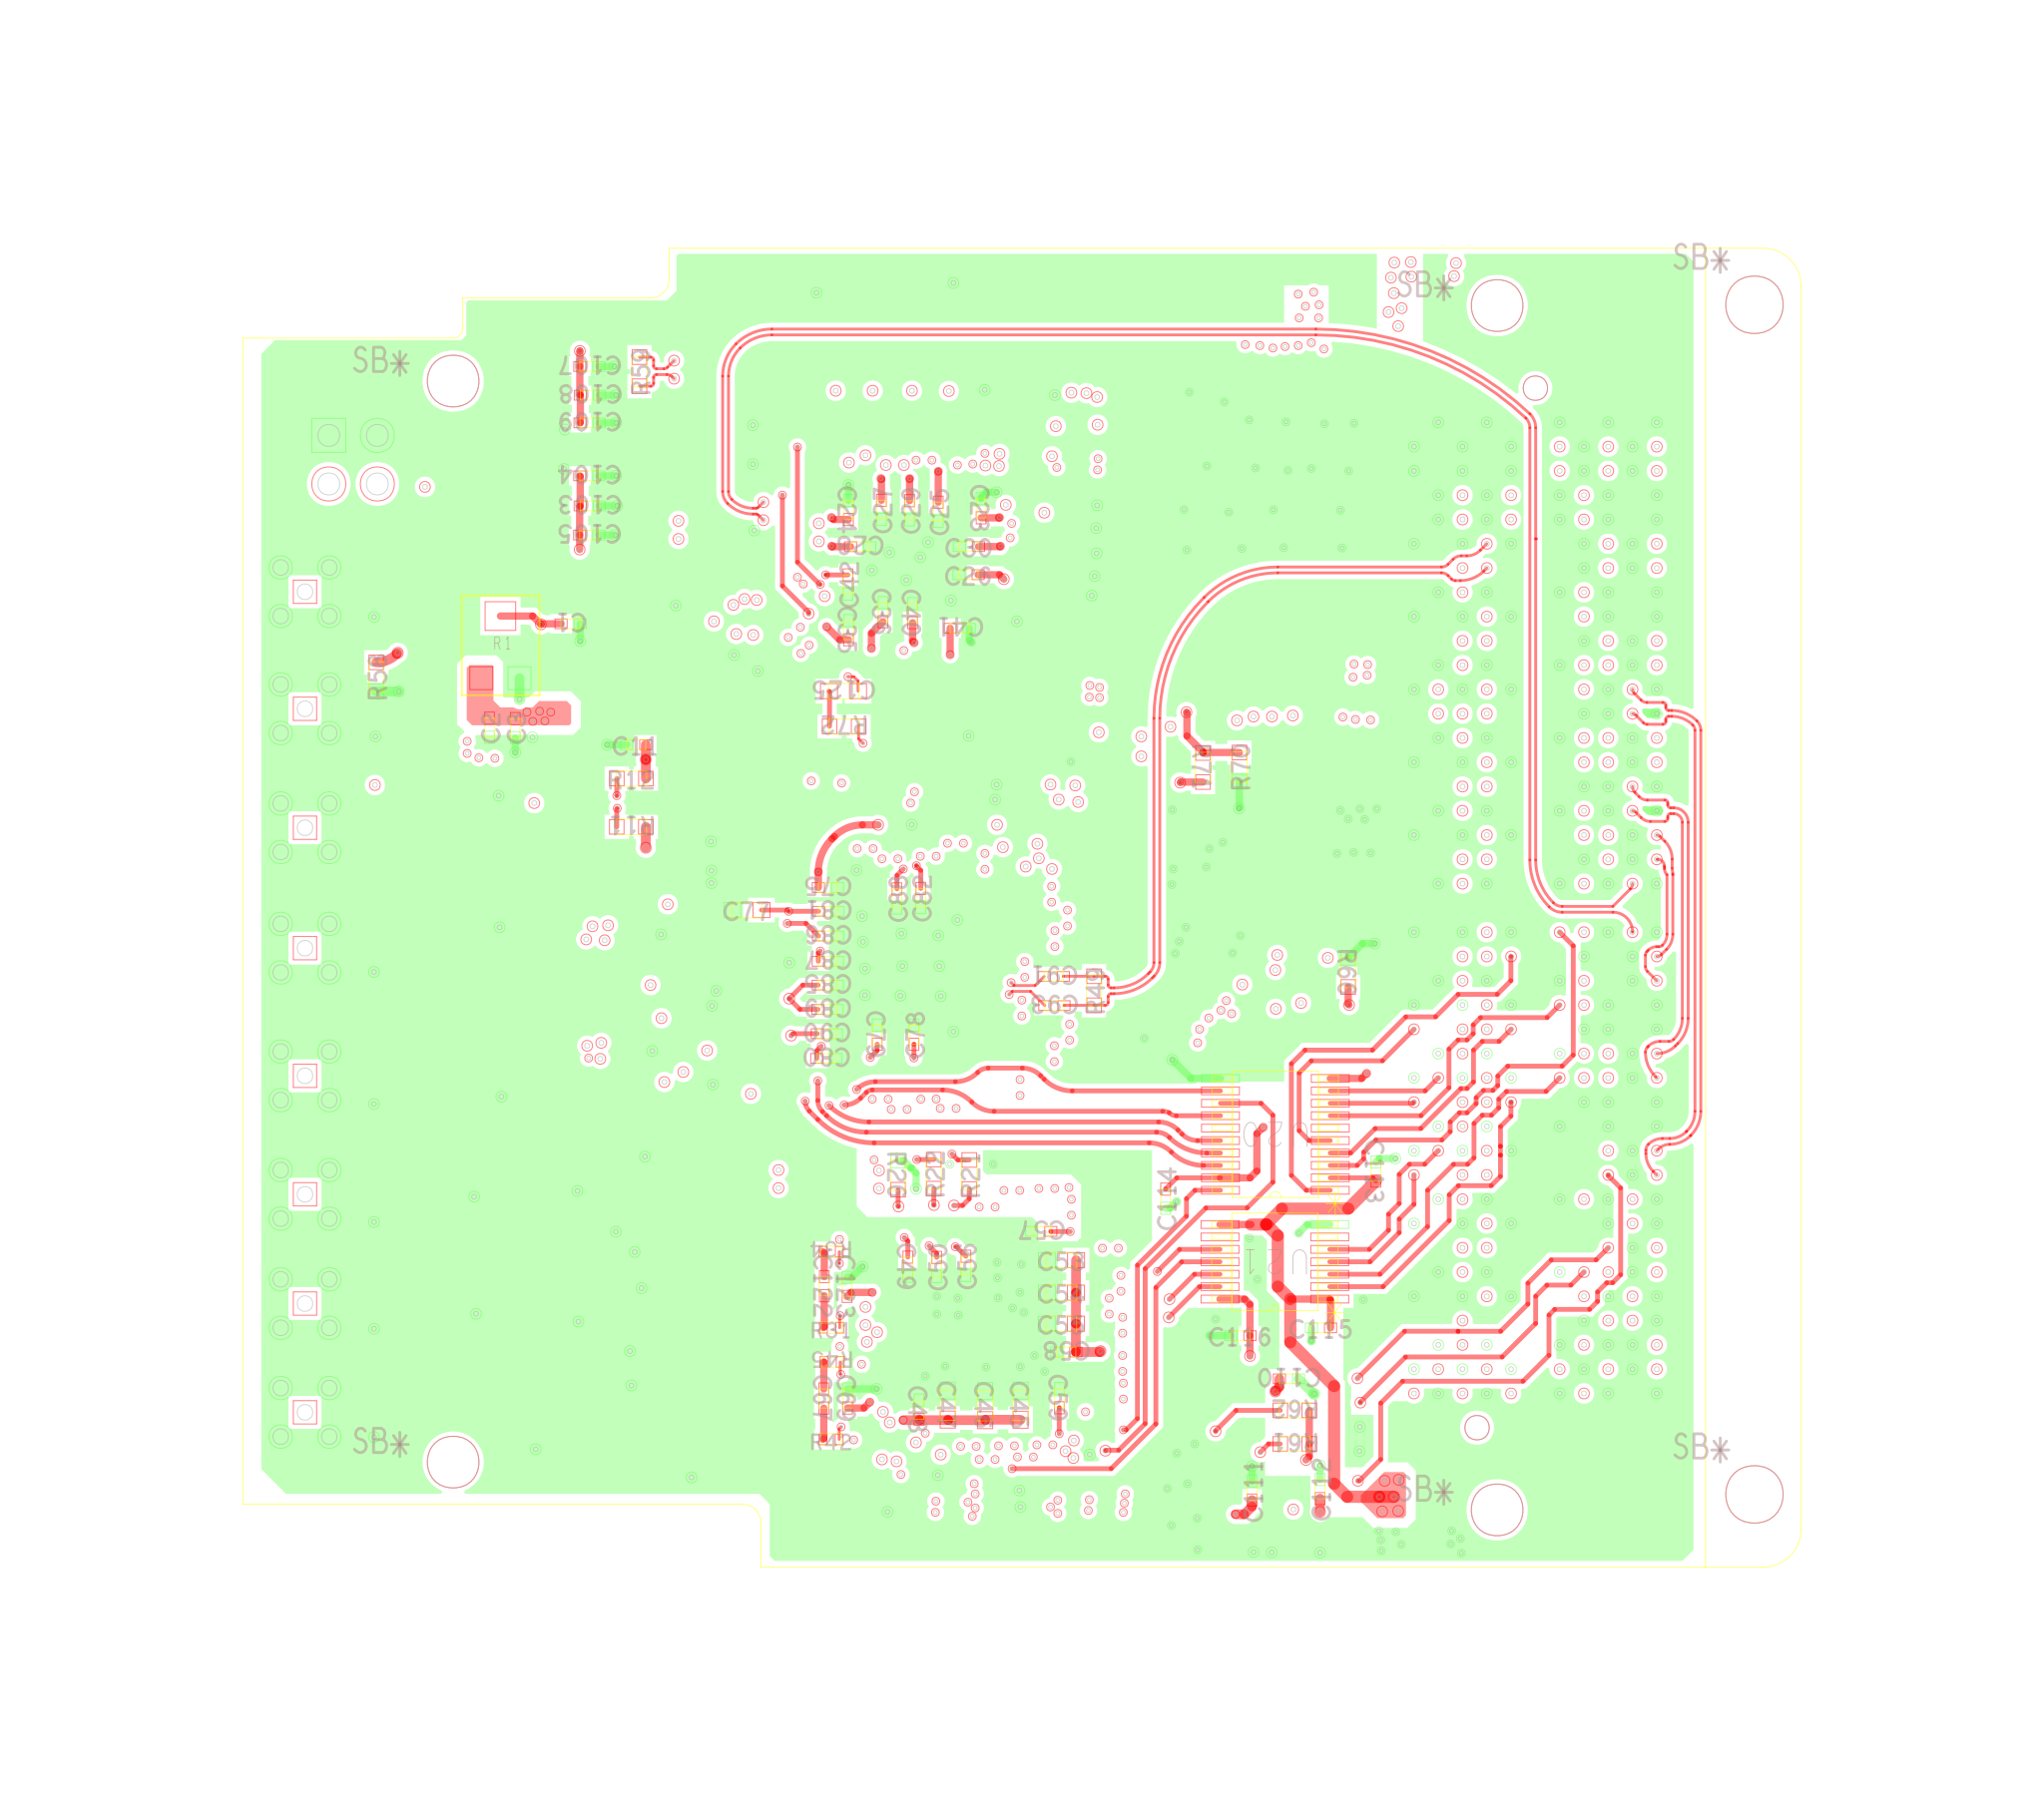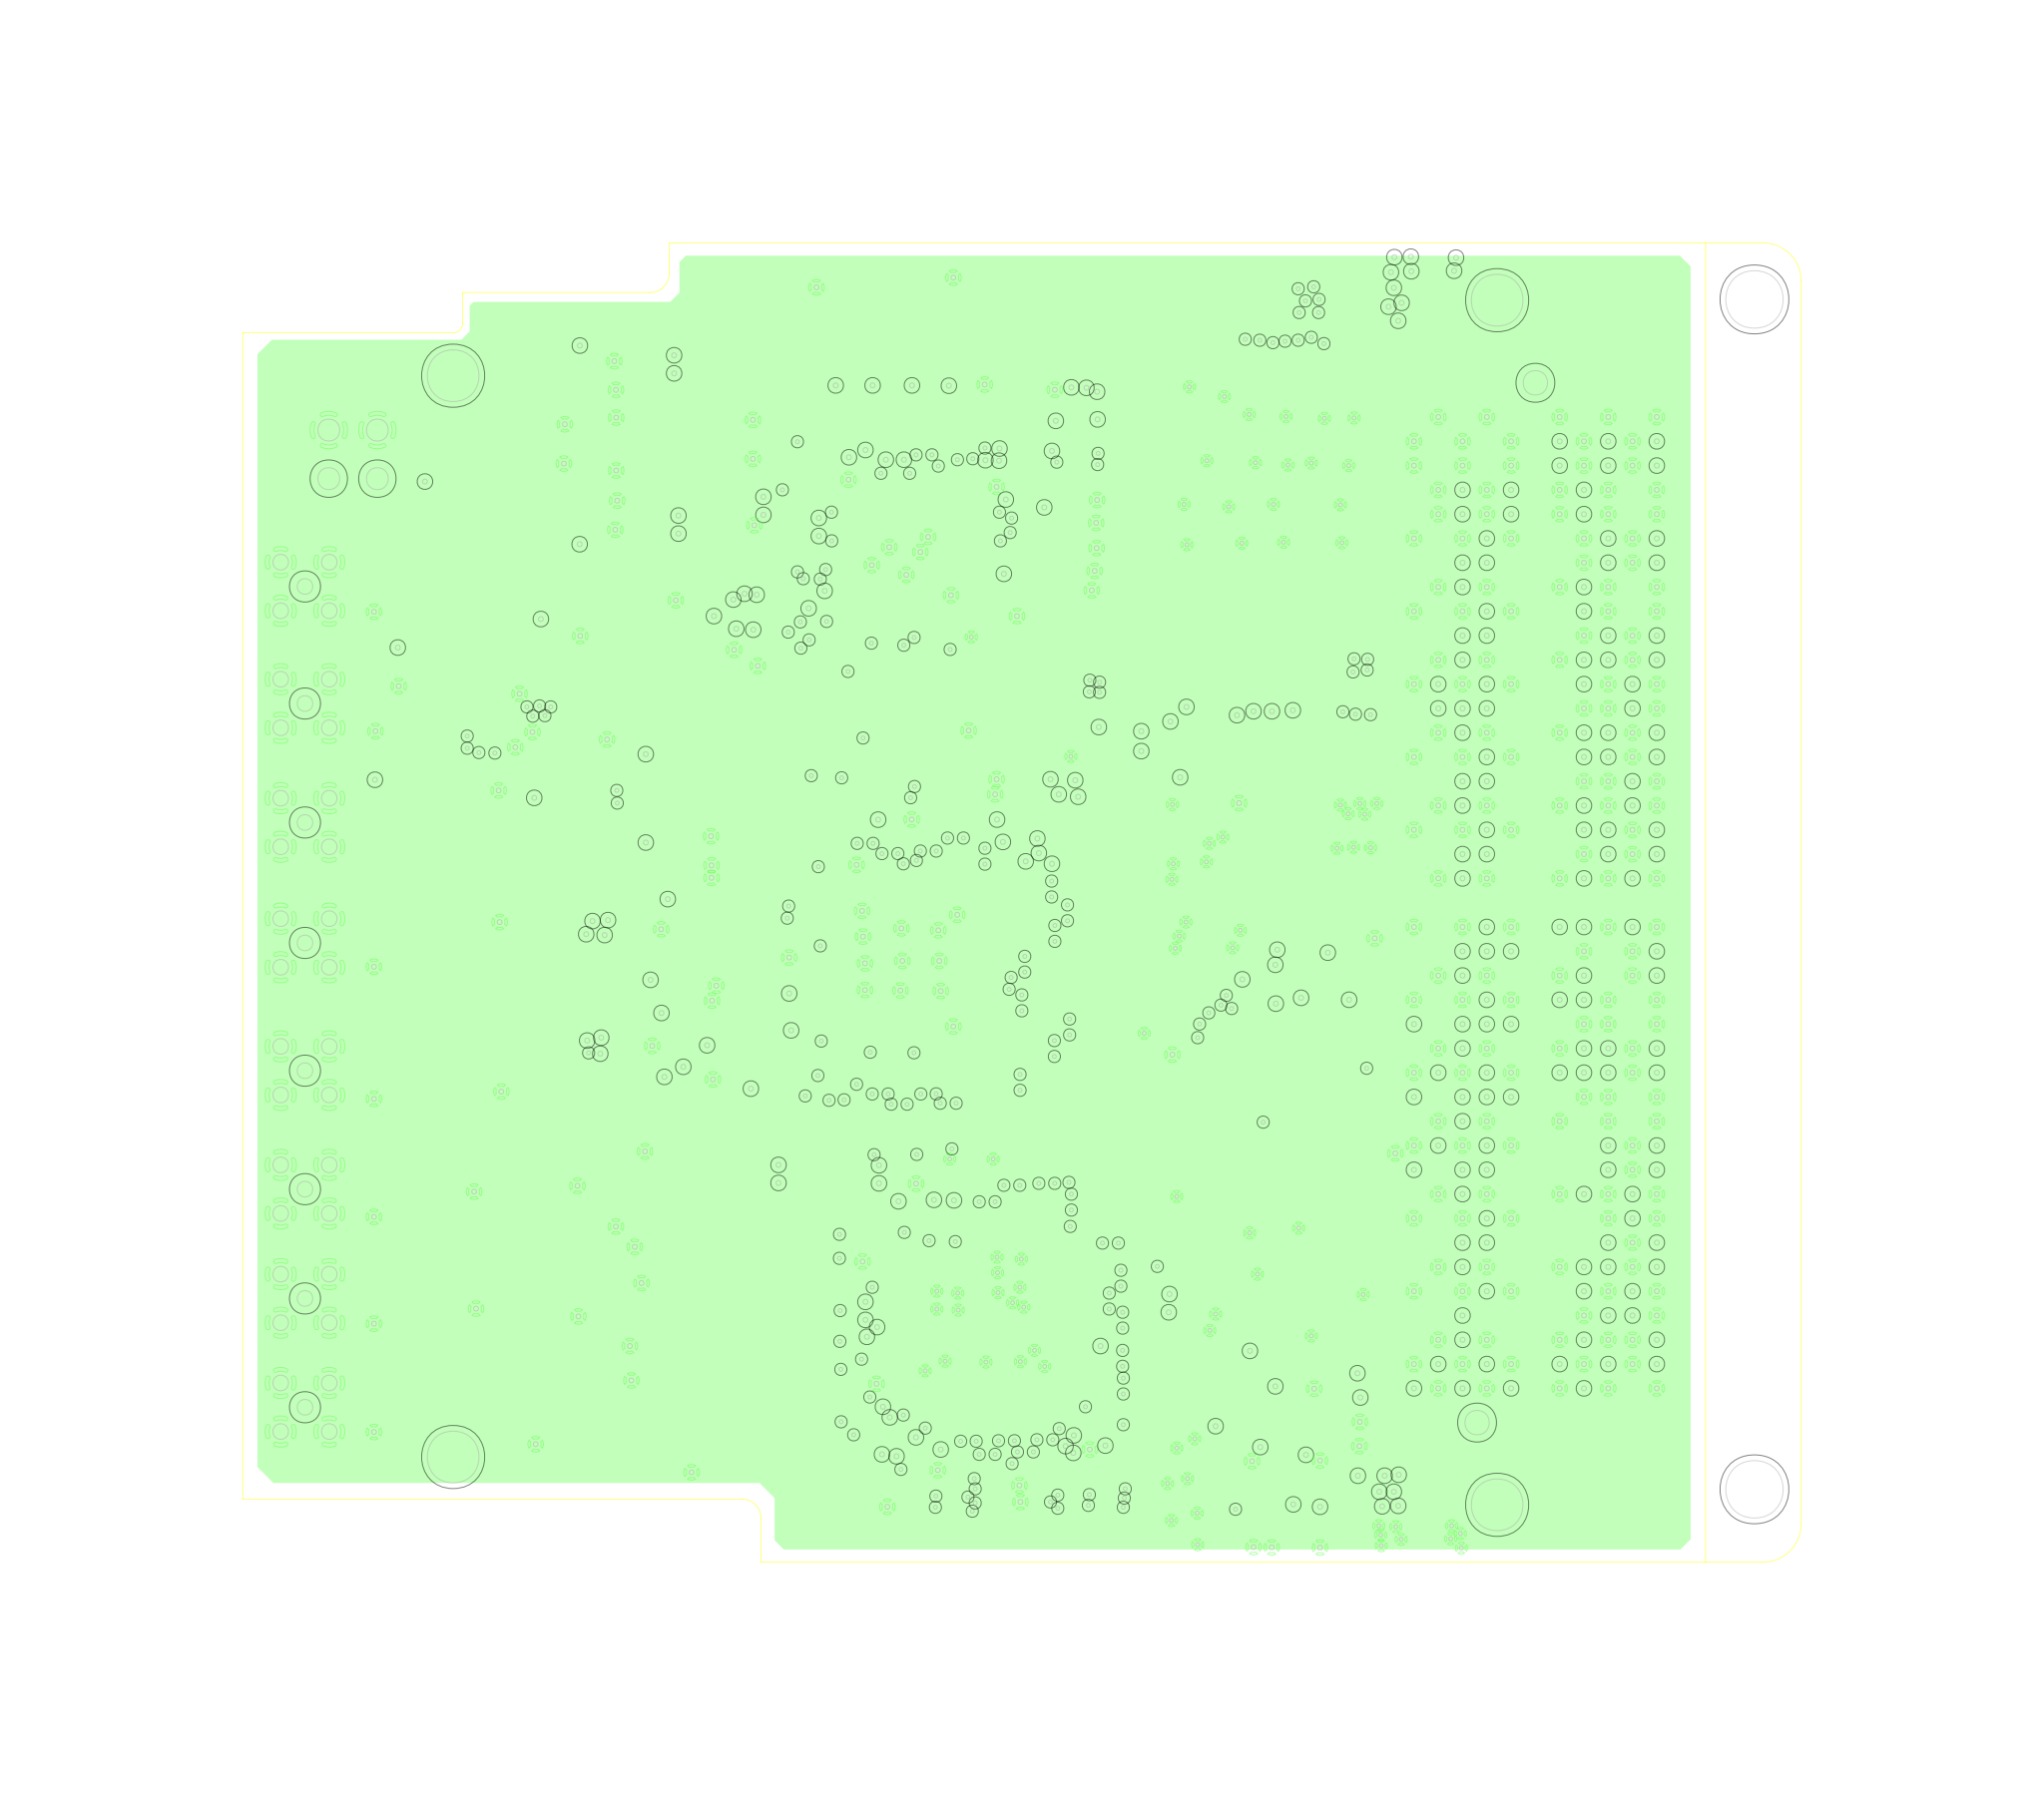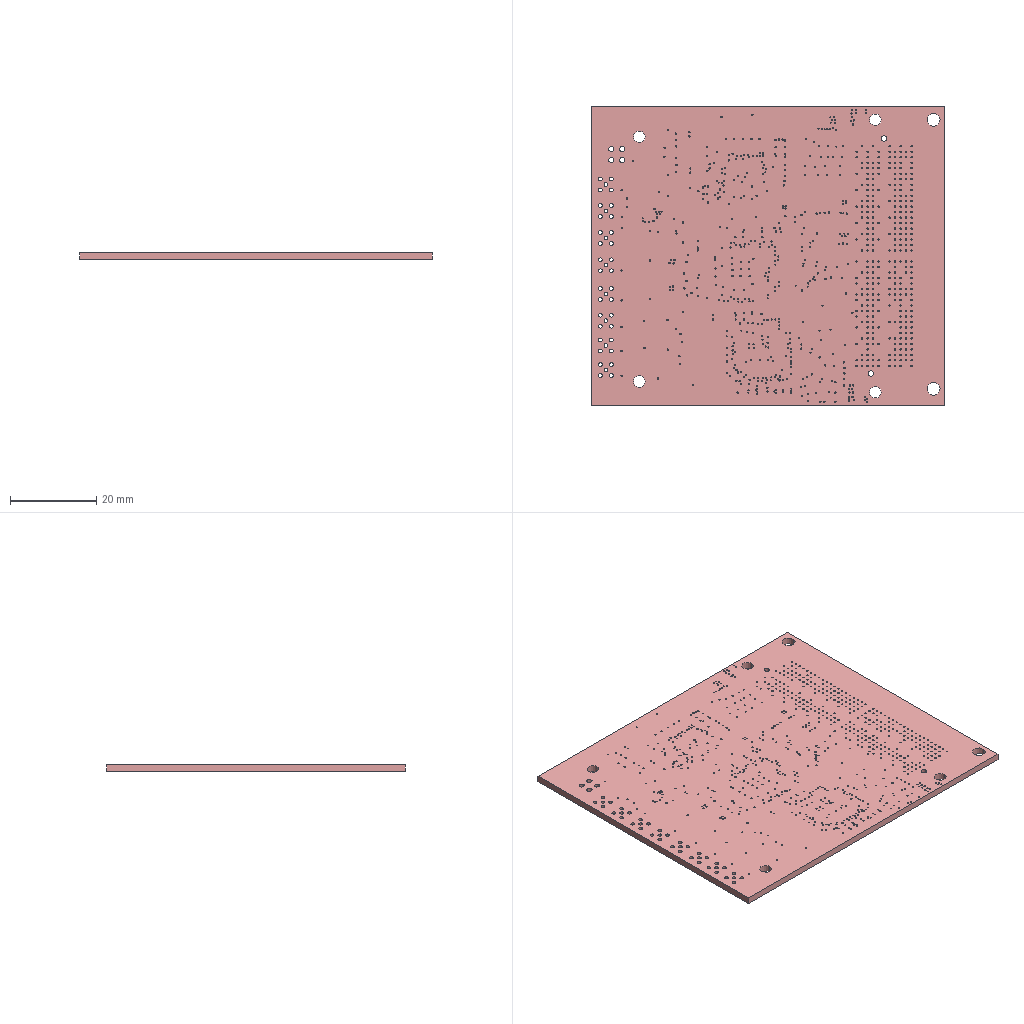Circuit board layout | Cadence Allegro | box 81.5 x 69 x 1.6 mm
Layer stack:
# Cadence Allegro layer stack of  (unit mm; from the constraint file cross-section; dielectric type: 0 not recorded (Allegro does not mark core vs prepreg), 3 surface material)
index,name,kind,layer,copper_thickness_mm,dielectric_type,dielectric_thickness_mm,dielectric_material,dielectric_constant
0,Top Surface,other,,,,,,
1,TOP,copper,TOP,0.0305,,,,
2,Dielectric1,dielectric,,,0,0.2032,FR-4,4.5
3,GND02,copper,GND02,0.0305,,,,
4,Dielectric2,dielectric,,,0,0.2032,FR-4,4.5
5,ART03,copper,ART03,0.0305,,,,
6,Dielectric3,dielectric,,,0,0.2032,FR-4,4.5
7,GND04,copper,GND04,0.0305,,,,
8,Dielectric4,dielectric,,,0,0.2032,FR-4,4.5
9,PWR05,copper,PWR05,0.0305,,,,
10,Dielectric5,dielectric,,,0,0.2032,FR-4,4.5
11,ART06,copper,ART06,0.0305,,,,
12,Dielectric6,dielectric,,,0,0.2032,FR-4,4.5
13,GND07,copper,GND07,0.0305,,,,
14,Dielectric7,dielectric,,,0,0.2032,FR-4,4.5
15,BOTTOM,copper,BOTTOM,0.0305,,,,
16,Bottom Surface,other,,,,,,
# drill layer pairs: low layer,high layer
drill_pair,TOP,BOTTOM
Part placement:
REFDES,COMP_VALUE,SYM_NAME,SYM_X,SYM_Y,SYM_ROTATE,SYM_MIRROR
C1,100nF,FPC-0402C,2831.000,3523.000,180.000,NO
C2,1uF,FPC-0402C,2664.000,3309.000,90.000,NO
C3,100nF,FPC-0402C,2717.000,3308.000,90.000,NO
C4,10nF,FPC-0402C,2716.000,3309.000,270.000,YES
C10,100nF,FPC-0402C,2426.240,2935.189,270.000,YES
C11,100nF,FPC-0402C,2966.000,3274.000,0.000,NO
C12,10uF,FPC-0603C,3650.559,3358.776,90.000,YES
C13,10uF,FPC-0603C,3236.177,3890.441,0.000,YES
C14,1uF,FPC-0402C,3236.177,3388.083,0.000,YES
C15,100nF,FPC-0402C,2954.913,3104.917,180.000,YES
C18,100nF,FPC-0402C,2957.181,3200.917,180.000,YES
C19,100nF,FPC-0402C,2426.240,3122.441,90.000,YES
C20,10uF,FPC-0603C,3836.142,3784.441,0.000,YES
C21,47uF,FPC-1206C,3766.240,3920.307,270.000,YES
C22,10uF,FPC-0603C,3683.559,3941.394,90.000,YES
C23,100nF,FPC-0402C,3676.083,3760.953,270.000,NO
C24,100nF,FPC-0402C,3403.083,3757.575,270.000,NO
C25,100nF,FPC-0402C,3587.917,3753.803,90.000,NO
C26,100nF,FPC-0402C,3650.315,3624.083,0.000,NO
C27,100nF,FPC-0402C,3470.917,3757.717,90.000,NO
C28,100nF,FPC-0402C,3427.063,3681.917,180.000,NO
C29,100nF,FPC-0402C,3528.917,3756.850,90.000,NO
C30,100nF,FPC-0402C,3651.071,3682.083,0.000,NO
C31,10uF,FPC-0603C,3836.142,3447.441,0.000,YES
C32,100nF,FPC-0402C,3834.142,3560.083,0.000,YES
C33,100nF,FPC-0402C,3834.142,3508.083,0.000,YES
C34,10uF,FPC-0603C,3239.177,3458.559,180.000,YES
C35,100nF,FPC-0402C,3403.083,3509.823,270.000,NO
C36,100nF,FPC-0402C,3474.000,3547.000,270.000,NO
C37,1uF,FPC-0603C,3393.980,3384.740,0.000,YES
C38,10nF,FPC-0603C,3535.823,3420.260,180.000,YES
C39,10uF,FPC-0603C,3239.177,3683.559,180.000,YES
C40,100nF,FPC-0402C,3535.083,3545.039,270.000,NO
C41,100nF,FPC-0402C,3632.055,3513.917,180.000,NO
C42,100nF,FPC-0402C,3401.917,3603.992,90.000,NO
C43,10uF,FPC-0603C,3618.559,1739.516,90.000,YES
C44,100nF,FPC-0402C,3483.083,1749.094,270.000,YES
C45,10uF,FPC-0603C,3757.441,1913.673,270.000,NO
C46,10uF,FPC-0603C,3684.441,1912.831,270.000,NO
C47,10uF,FPC-0603C,3607.441,1913.988,270.000,NO
C48,10nF,FPC-0402C,3548.240,1904.433,270.000,NO
C49,10nF,FPC-0402C,3525.240,2199.008,270.000,NO
C50,10nF,FPC-0402C,3584.760,2198.370,90.000,NO
C51,10uF,FPC-0603C,3934.559,1738.146,90.000,YES
C52,100nF,FPC-0402C,3788.083,1748.472,270.000,YES
C53,10uF,FPC-0603C,3841.697,2212.441,0.000,NO
C54,10uF,FPC-0603C,3841.539,2145.441,0.000,NO
C55,10uF,FPC-0603C,3841.382,2081.441,0.000,NO
C56,10nF,FPC-0402C,3644.760,2200.748,90.000,NO
C57,10nF,FPC-0402C,3799.874,2271.760,180.000,NO
C58,10nF,FPC-0402C,3851.496,2023.260,180.000,NO
C59,10nF,FPC-0402C,3837.240,1928.118,270.000,NO
C60,100nF,FPC-0402C,2426.240,2198.748,270.000,YES
C61,100nF,FPC-0402C,3292.083,2105.228,270.000,YES
C62,100nF,FPC-0402C,3291.917,2200.811,90.000,YES
C63,100nF,FPC-0402C,2904.433,2300.083,0.000,YES
C64,100nF,FPC-0402C,2904.016,2354.917,180.000,YES
C65,100nF,FPC-0402C,2426.240,1976.323,270.000,YES
C66,100nF,FPC-0402C,3293.083,1876.701,270.000,YES
C67,3.3pF,FPC-0402C,3352.240,1927.433,270.000,NO
C68,100nF,FPC-0402C,3292.917,1971.921,90.000,YES
C69,100nF,FPC-0402C,3401.083,1927.543,270.000,NO
C70,100nF,FPC-0402C,2896.165,2025.083,0.000,YES
C71,100nF,FPC-0402C,2896.213,2085.917,180.000,YES
C72,100nF,FPC-0402C,3406.409,2349.083,0.000,YES
C73,100nF,FPC-0402C,3407.031,2408.083,0.000,YES
C74,10uF,FPC-0603C,3569.441,3139.122,270.000,YES
C75,100nF,FPC-0402C,3360.654,2979.917,180.000,NO
C76,47uF,FPC-1206C,3172.504,2933.240,0.000,YES
C77,10uF,FPC-0603C,3193.965,2933.441,0.000,NO
C78,100nF,FPC-0402C,3537.917,2676.724,90.000,NO
C79,100nF,FPC-0402C,3462.083,2676.898,270.000,NO
C80,100nF,FPC-0402C,3357.520,2627.917,180.000,NO
C81,100nF,FPC-0402C,3361.142,2930.917,180.000,NO
C82,100nF,FPC-0402C,3551.917,2958.236,90.000,NO
C83,10uF,FPC-0603C,3744.559,3139.193,90.000,YES
C84,10uF,FPC-0603C,3671.559,3139.350,90.000,YES
C85,100nF,FPC-0402C,3360.386,2778.917,180.000,NO
C86,100nF,FPC-0402C,3361.126,2880.059,180.000,NO
C87,100nF,FPC-0402C,3360.630,2827.917,180.000,NO
C88,100nF,FPC-0402C,3502.760,2957.378,90.000,NO
C89,100nF,FPC-0402C,3359.874,2728.917,180.000,NO
C90,100nF,FPC-0402C,3358.496,2678.917,180.000,NO
C91,10nF,FPC-0402C,3825.740,2796.760,180.000,NO
C92,10nF,FPC-0402C,3327.240,3150.638,270.000,YES
C93,10nF,FPC-0402C,3826.984,2736.760,180.000,NO
C94,10nF,FPC-0402C,3387.240,3147.394,270.000,YES
C95,100nF,FPC-0402C,3180.118,2736.083,0.000,YES
C96,100nF,FPC-0402C,2426.240,2424.260,270.000,YES
C97,1nF,FPC-0402C,3171.008,3014.760,180.000,YES
C98,150nF,FPC-0402C,3170.772,3074.760,180.000,YES
C99,100nF,FPC-0402C,2941.362,2643.083,0.000,YES
C100,100nF,FPC-0402C,2426.240,2672.591,270.000,YES
C101,100nF,FPC-0402C,2957.787,2883.240,0.000,YES
C102,100nF,FPC-0402C,2429.760,3426.165,90.000,YES
C103,1uF,FPC-0402C,2870.386,3765.760,180.000,NO
C104,100nF,FPC-0402C,2869.543,3827.760,180.000,NO
C105,100nF,FPC-0402C,2869.244,3705.760,180.000,NO
C106,100nF,FPC-0402C,2426.240,3664.701,270.000,YES
C107,1uF,FPC-0402C,2869.606,4052.917,180.000,NO
C108,100nF,FPC-0402C,2870.677,3993.760,180.000,NO
C109,100nF,FPC-0402C,2870.055,3936.760,180.000,NO
C110,100nF,FPC-0402C,4310.000,1968.000,180.000,NO
C111,100nF,FPC-0402C,4234.000,1738.000,90.000,NO
C112,100nF,FPC-0402C,4374.000,1741.000,90.000,NO
C113,100nF,FPC-0402C,4489.000,2395.000,270.000,NO
C114,100nF,FPC-0402C,4056.000,2339.000,90.000,NO
C115,100nF,FPC-0402C,4376.000,2073.000,0.000,NO
C116,100nF,FPC-0402C,4210.000,2057.000,0.000,NO
C117,100uF,FPC-3528T,4184.000,4187.000,0.000,YES
C118,330uF,FPC-7343T,4303.000,3100.000,90.000,YES
C119,10uF,FPC-0603C,4150.000,2799.000,90.000,YES
C120,33pF,FPC-0402C,4336.000,2811.000,270.000,YES
C121,10uF,FPC-0603C,4246.000,2801.000,90.000,YES
C122,3.3pF,FPC-0402C,3353.240,2158.811,270.000,NO
C123,100nF,FPC-0402C,3400.083,2157.465,270.000,NO
C124,10uF,FPC-0603C,4459.000,3219.000,270.000,YES
C125,1uF,FPC-0603C,3392.823,3384.260,180.000,NO
C126,1nF,FPC-0402C,3182.370,2581.240,0.000,YES
C127,47uF,FPC-1206C,4144.000,3191.000,90.000,YES
C128,47uF,FPC-1206C,4594.000,1696.000,90.000,YES
C129,10nF,FPC-0603C,3535.823,3354.260,180.000,YES
C130,1nF,FPC-1206C,3559.000,4162.000,0.000,YES
C134,1nF,FPC-1206C,3020.000,1823.000,0.000,YES
D2,533-0121F,FPC-LED4-4R3X8R1-1R1-1,2383.000,3861.000,90.000,YES
D3,PESD3V3X1BL,SOD882,2426.043,2828.339,270.000,YES
D4,PESD3V3X1BL,SOD882,2426.043,2096.535,270.000,YES
D5,PESD3V3X1BL,SOD882,2426.043,1872.559,270.000,YES
D6,PESD3V3X1BL,SOD882,2426.043,2320.583,270.000,YES
D7,PESD3V3X1BL,SOD882,2426.043,2566.606,270.000,YES
D8,PESD3V3X1BL,SOD882,2429.000,3321.000,270.000,YES
D9,PESD3V3X1BL,SOD882,2426.043,3561.654,270.000,YES
J1,CON-MMCX-Angle,SMA,2284.000,2855.000,0.000,YES
J2,CON-MMCX,SMA,2284.000,3103.000,0.000,YES
J3,CON-MMCX-Angle,SMA,2284.000,2123.000,0.000,YES
J4,CON-MMCX-Angle,SMA,2284.000,1899.000,0.000,YES
J5,CON-MMCX-Angle,SMA,2284.000,2348.000,0.000,YES
J6,CON-MMCX-Angle,SMA,2284.000,2592.000,0.000,YES
J7,CON-MMCX-Angle,SMA,2284.000,3348.000,0.000,YES
J8,CON-MMCX-Angle,SMA,2284.000,3589.000,0.000,YES
J9,ASP-134485-01,FPC-CON90VP1R27-10X40SM,4817.421,2937.870,270.000,YES
L1,BLM18HE152SN1,FPC-0603L,2647.000,3309.000,270.000,YES
L2,BLM18HE152SN1,FPC-0603L,3836.142,3377.240,0.000,YES
L3,BLM18HE152SN1,FPC-0603L,3239.177,3530.760,180.000,YES
L4,BLM18HE152SN1,FPC-0603L,3239.177,3609.760,180.000,YES
L6,BLM18HE152SN1,FPC-0603L,3494.760,3138.858,90.000,YES
L12,BLM18EG221SN1,FPC-0603L,3843.858,3109.240,0.000,YES
L13,BLM18EG221SN1,FPC-0603L,3548.240,1739.142,270.000,YES
L14,BLM18HE152SN1,FPC-0603L,3862.240,1738.142,270.000,YES
L15,BLM18EG221SN1,FPC-0603L,3871.760,3889.858,90.000,YES
R1,10K,VR5,2647.000,3411.000,0.000,NO
R2,33R,FPC-0603R,3126.000,3451.000,270.000,YES
R3,4.7K,FPC-0603R,2850.000,3313.000,180.000,YES
R11,121R,FPC-0603R,2955.835,3104.760,180.000,NO
R12,121R,FPC-0603R,2956.008,3204.240,0.000,NO
R13,NC_10K,FPC-0603R,3836.142,3627.240,0.000,YES
R14,4.7K,FPC-0603R,3452.760,3941.394,90.000,YES
R15,1K,FPC-0603R,3376.760,3941.394,90.000,YES
R16,1K,FPC-0603R,3836.142,3704.240,0.000,YES
R17,33R,FPC-0603R,3609.760,3941.394,90.000,YES
R18,200R,FPC-0603R,3835.291,3310.760,180.000,YES
R19,4.7K,FPC-0603R,3533.760,3941.394,90.000,YES
R20,10K,FPC-0603R,3393.866,3311.240,0.000,YES
R21,NC_0R,FPC-0603R,3651.760,2388.819,90.000,NO
R22,NC_0R,FPC-0603R,3578.760,2389.661,90.000,NO
R23,NC_0R,FPC-0603R,3505.240,2388.504,270.000,YES
R24,0R,FPC-0603R,3650.760,2389.126,90.000,YES
R25,0R,FPC-0603R,3577.760,2390.283,90.000,YES
R26,0R,FPC-0603R,3505.240,2387.441,270.000,NO
R28,5R,FPC-0402R,3369.209,2124.760,180.000,YES
R29,NC_49.9R,FPC-0603R,2897.772,2229.240,0.000,YES
R30,24.9R,FPC-0402R,3368.594,2072.240,0.000,YES
R31,49.9R,FPC-0402R,3368.232,2073.240,0.000,NO
R32,NC_49.9R,FPC-0603R,2903.071,2425.760,180.000,YES
R33,24.9R,FPC-0402R,3367.862,2229.760,180.000,YES
R34,49.9R,FPC-0402R,3367.311,2229.760,180.000,NO
R36,5R,FPC-0402R,3367.665,2179.760,180.000,YES
R37,4.7K,FPC-0603R,3708.240,1738.220,270.000,YES
R39,5R,FPC-0402R,3371.122,1895.760,180.000,YES
R40,NC_49.9R,FPC-0603R,2888.087,1954.240,0.000,YES
R41,24.9R,FPC-0402R,3371.681,1842.240,0.000,YES
R42,49.9R,FPC-0402R,3367.146,1843.240,0.000,NO
R43,NC_49.9R,FPC-0603R,2898.756,2154.760,180.000,YES
R44,24.9R,FPC-0402R,3370.776,2003.760,180.000,YES
R45,49.9R,FPC-0402R,3369.272,2002.760,180.000,NO
R47,5R,FPC-0402R,3370.579,1952.760,180.000,YES
R48,100R,FPC-0603R,3323.240,2378.378,270.000,YES
R49,100R,FPC-0603R,3908.760,2767.220,90.000,NO
R50,100R,FPC-0603R,3356.937,3065.240,0.000,YES
R51,953R,FPC-0603R,3168.961,2800.760,180.000,YES
R52,100R,FPC-0603R,2950.906,2710.760,180.000,YES
R53,93.1R,FPC-0603R,3265.240,3043.803,270.000,YES
R54,100R,FPC-0603R,2956.252,2579.240,0.000,YES
R55,100R,FPC-0603R,2965.591,2819.760,180.000,YES
R56,100R,FPC-0603R,2965.567,2945.240,0.000,YES
R57,1K,FPC-0603R,3172.079,2644.240,0.000,YES
R58,49.9R,FPC-0603R,2430.760,3413.646,90.000,NO
R59,100R,FPC-0603R,2972.760,4042.276,90.000,NO
R60,4.7K,FPC-0603R,4604.000,4206.000,270.000,YES
R61,4.7K,FPC-0603R,4322.000,1834.000,180.000,NO
R62,4.7K,FPC-0603R,4322.000,1903.000,180.000,NO
R63,100R,FPC-0603R,2534.000,3868.000,90.000,YES
R64,1K,FPC-0603R,3236.177,3819.760,180.000,YES
R65,NC_14K,FPC-0603R,4432.000,2805.000,270.000,YES
R66,NC_30.1K,FPC-0603R,4432.000,2805.000,270.000,NO
R67,NC_0R,FPC-0603R,4443.654,4103.240,0.000,YES
R68,NC_0R,FPC-0603R,4444.000,4170.000,0.000,YES
R69,NC_0R,FPC-0603R,4444.000,4236.000,0.000,YES
R70,30.1K,FPC-0603R,4208.000,3228.000,90.000,NO
R71,51K,FPC-0603R,4133.000,3227.000,270.000,NO
R72,10K,FPC-0603R,3394.024,3311.760,180.000,NO
R73,1M,FPC-0603R,3367.000,4162.000,0.000,YES
R74,1M,FPC-0603R,2841.000,1823.000,0.000,YES
T1,TC4-1W+,FPC-TRAN5SM-3R81X3R81,2745.382,3153.740,270.000,YES
T2,TC1-1T+,FPC-TRAN5SM-3R81X3R81,2694.839,2324.535,270.000,YES
T3,TC1-1T+,FPC-TRAN5SM-3R81X3R81,3090.161,2320.945,90.000,YES
T4,TC1-1T+,FPC-TRAN5SM-3R81X3R81,2698.839,2088.575,270.000,YES
T5,TC1-1T+,FPC-TRAN5SM-3R81X3R81,3085.161,2044.906,90.000,YES
T6,TC4-1T+,FPC-TRAN5SM-3R81X3R81,2750.839,2643.614,270.000,YES
T7,TC4-1T+,FPC-TRAN5SM-3R81X3R81,2747.382,2884.220,270.000,YES
U5,CDCE62005RGZ,FPC-QFN7X7-48-1,3538.839,3653.358,270.000,YES
U10,ADS62P29IRGCT,FPC-QFN9X9-64-1,3689.169,2078.390,270.000,YES
U14,DAC5682ZIRGCT,FPC-QFN9X9-64-1,3508.331,2791.331,90.000,YES
U15,DS90LV017ATM,FPC-SO8-150,2873.000,3767.000,180.000,YES
U16,DS90LV018ATM,FPC-SO8-150,2873.000,3998.000,0.000,YES
U17,AT24C128BN-SH-B,FPC-SO8-150,4307.000,1894.000,0.000,YES
U18,AD7415ARTZ,FPC-SOT23-6,4237.083,1696.961,270.000,YES
U19,AD7415ARTZ,FPC-SOT23-6,4374.000,1697.000,270.000,YES
U20,TXB0108PWR,FPC-TSSOP20-0R65-4R40,4282.000,2471.500,180.000,NO
U21,TXS0104EPWR,FPC-TSSOP14-0R65-4R40,4281.000,2209.000,180.000,NO
U22,TPS78601KTT,FPC-TO-263,4300.000,2237.000,180.000,YES
U23,TPS75801KTT_3A,FPC-TO-263,4270.500,3823.500,0.000,YES
X1,TAITIEN_TCXO_TS_10Mhz,FPC-CO10-5R0X7R0-S,3047.500,3373.500,0.000,YES
Pad and via stacks:
# Allegro (Cadence) via spans and padstacks; design units: ("mils" 3 1000)
# via spans: padstack,start_layer,end_layer,net_example,count
VIA8-F,ETCH/TOP,ETCH/BOTTOM,VCC_3.3V,288
VIA10,ETCH/TOP,ETCH/BOTTOM,ADC_OF,15
VIA10-F,ETCH/TOP,ETCH/BOTTOM,DGND,527
# Allegro padstack definitions: name,start_layer,end_layer,drill,plating,holeType,type
SMD1R60X2R70,"ETCH/TOP","ETCH/TOP",0.0,"PLATED","none","smd"
SMD2R00X2R20,"ETCH/TOP","ETCH/TOP",0.0,"PLATED","none","smd"
SMD2R60X2R20,"ETCH/TOP","ETCH/TOP",0.0,"PLATED","none","smd"
SMD0R51X0R51,"ETCH/TOP","ETCH/TOP",0.0,"PLATED","none","smd"
SMD40_50,"ETCH/TOP","ETCH/TOP",0.0,"PLATED","none","smd"
SMD0R76X0R80,"ETCH/TOP","ETCH/TOP",0.0,"PLATED","none","smd"
SMD1R00X4R50,"ETCH/TOP","ETCH/TOP",0.0,"PLATED","none","smd"
SMD10R50X10R80,"ETCH/TOP","ETCH/TOP",0.0,"NON_PLATED","none","smd"
SMDF1R80X0R40,"ETCH/TOP","ETCH/TOP",0.0,"NON_PLATED","none","smd"
SMD15_80OB,"ETCH/TOP","ETCH/TOP",0.0,"PLATED","none","smd"
SMD80_20,"ETCH/TOP","ETCH/TOP",0.0,"PLATED","none","smd"
SMD32_10OB,"ETCH/TOP","ETCH/TOP",0.0,"PLATED","none","smd"
SMD220_220,"ETCH/TOP","ETCH/TOP",0.0,"PLATED","none","smd"
SMDC0R64,"ETCH/TOP","ETCH/TOP",0.0,"PLATED","none","smd"
BALL25,"ETCH/TOP","ETCH/TOP",0.0,"PLATED","none","smd"
FPC-MARK1R0S,"ETCH/TOP","ETCH/TOP",0.0,"PLATED","none","smd"
SMD24_32,"ETCH/TOP","ETCH/TOP",0.0,"PLATED","none","smd"
VIA10-F,"ETCH/TOP","ETCH/BOTTOM",10.0,"PLATED","circle_drill","through"
VIA8-F,"ETCH/TOP","ETCH/BOTTOM",8.0,"PLATED","circle_drill","through"
PAD50CIR50U,"ETCH/TOP","ETCH/BOTTOM",50.0,"NON_PLATED","circle_drill","through"
PAD63CIR63U,"ETCH/TOP","ETCH/BOTTOM",63.0,"NON_PLATED","circle_drill","through"
PAD80SQ42D,"ETCH/TOP","ETCH/BOTTOM",42.0,"PLATED","circle_drill","through"
PAD60CIR40D,"ETCH/TOP","ETCH/BOTTOM",40.0,"PLATED","circle_drill","through"
PAD80SQ38D,"ETCH/TOP","ETCH/BOTTOM",38.0,"PLATED","circle_drill","through"
PAD52CIR32D,"ETCH/TOP","ETCH/BOTTOM",32.0,"PLATED","circle_drill","through"
PAD60SQ40D,"ETCH/TOP","ETCH/BOTTOM",40.0,"PLATED","circle_drill","through"
THC0R00D2R70,"ETCH/TOP","ETCH/BOTTOM",106.299,"NON_PLATED","circle_drill","through"
VIA10,"ETCH/TOP","ETCH/BOTTOM",10.0,"PLATED","circle_drill","through"
THC0R00D3R00,"ETCH/TOP","ETCH/BOTTOM",118.11,"NON_PLATED","circle_drill","through"
OBL11X39,"ETCH/TOP","ETCH/TOP",0.0,"PLATED","none","smd"
S220_NP,"ETCH/TOP","ETCH/TOP",0.0,"PLATED","none","smd"
18C10VIA_18INL,"ETCH/TOP","ETCH/BOTTOM",10.0,"PLATED","circle_drill","through"
SMD_SQ30,"ETCH/TOP","ETCH/TOP",0.0,"PLATED","none","smd"
RECT22X16,"ETCH/TOP","ETCH/TOP",0.0,"PLATED","none","smd"
SMD1_2X1_2,"ETCH/TOP","ETCH/TOP",0.0,"PLATED","none","smd"
SMD1_6X1_5,"ETCH/TOP","ETCH/TOP",0.0,"PLATED","none","smd"
TH47_CR70,"ETCH/TOP","ETCH/BOTTOM",47.0,"PLATED","circle_drill","through"
TH63_CR95,"ETCH/TOP","ETCH/BOTTOM",63.0,"PLATED","circle_drill","through"
TH45_CR70,"ETCH/TOP","ETCH/BOTTOM",45.0,"PLATED","circle_drill","through"
TH45_SQ70,"ETCH/TOP","ETCH/BOTTOM",45.0,"PLATED","circle_drill","through"
RECT20X25,"ETCH/TOP","ETCH/TOP",0.0,"PLATED","none","smd"
RECT45X60,"ETCH/TOP","ETCH/TOP",0.0,"PLATED","none","smd"
RECT31X35,"ETCH/TOP","ETCH/TOP",0.0,"PLATED","none","smd"
RECT94X130,"ETCH/TOP","ETCH/TOP",0.0,"PLATED","none","smd"
SMD0_3X0_6,"ETCH/TOP","ETCH/TOP",0.0,"PLATED","none","smd"
RECT30X65,"ETCH/TOP","ETCH/TOP",0.0,"PLATED","none","smd"
SMD0_8X0_23,"ETCH/TOP","ETCH/TOP",0.0,"PLATED","none","smd"
SMD7_4X7_4,"ETCH/TOP","ETCH/TOP",0.0,"PLATED","none","smd"
SMD0_6X1_3,"ETCH/TOP","ETCH/TOP",0.0,"PLATED","none","smd"
RX46Y20D0T,"ETCH/TOP","ETCH/TOP",0.0,"NON_PLATED","none","smd"
RX78Y16D0T,"ETCH/TOP","ETCH/TOP",0.0,"NON_PLATED","none","smd"
RX40Y150D0T,"ETCH/TOP","ETCH/TOP",0.0,"NON_PLATED","none","smd"
RX420Y396D0T,"ETCH/TOP","ETCH/TOP",0.0,"NON_PLATED","none","smd"
SMD1_1X1_3,"ETCH/TOP","ETCH/TOP",0.0,"PLATED","none","smd"
SMD1_3X0_9,"ETCH/TOP","ETCH/TOP",0.0,"PLATED","none","smd"
SMD1_7X0_9,"ETCH/TOP","ETCH/TOP",0.0,"PLATED","none","smd"
TH32_CR48,"ETCH/TOP","ETCH/BOTTOM",32.0,"PLATED","circle_drill","through"
TH32_SQ48,"ETCH/TOP","ETCH/BOTTOM",32.0,"PLATED","circle_drill","through"
Design rules, without the lines most boards share, first 13 of 80 lines:
# Cadence Allegro design rules of  (from the Constraint Manager export constraints.dcfx, design unit mil; typed fields in mm)
# columns: name | kind | enabled | priority | scope1 | scope2 | descriptor | typed fields (field=value)
# Allegro precedence (priority 1 wins): 1 Region class-to-class, 2 Region class, 3 Region, 4 class-to-class, 5 DiffPair/Bus/NetGroup override, 6 NetClass, 7 constraint set (CSet) default
# per-layer values are written LAYER=value in the descriptor and LAYER:mm in the typed field; a maximum of 0 means no limit set
# --- net classes (and buses / net groups) ---
# (no net classes defined: every net uses the default constraint sets)
# --- track widths, neck and differential-pair gap (physical constraint sets) ---
DEFAULT | PhysicalCSet | enabled | 7 | Design default; Net(11): VCC_3.3V_IN, VCC_1.8V, VCC_12V, VCC_1.8V_A, VCC_IN, VCC_OUT, VCC_PLL, VCC_VCO, VCC_ADJ, VCC_3.3V, VCC_3.3V_TCXO | All | Physical Constraint (Min Line Width=10mil) (Max Line Width=0mil) (Min Neck Width=5mil) (Max Neck Length=0mil) (DiffPair Primary Gap=0mil) (DiffPair Neck Gap=0mil) (DiffPair Min Space=0mil) (DiffPair Coupled +Tol=0mil) (DiffPair Coupled -Tol=0mil) (Min BB Via Stagger=5mil) (Max BB Via Stagger=0mil) (T-junctions=ANYWHERE) (Pad-pad direct connect=NOT_ALLOWED) (Allowed vias=VIA8-F, VIA10-F, VIA10) | min_line_width=0.254 min_neck_width=0.127 min_bvia_stagger=0.127 max_bvia_stagger=0 ts_allowed=ANYWHERE diffp_primary_gap=0 diffp_neck_gap=0 max_line_width=0 maximum_neck_length=0 pad_pad_direct_connect=NOT_ALLOWED allow_on_etch_subclass=TRUE diffp_coupled_plus=0 diffp_coupled_minus=0 diffp_min_space=0 vias=VIA8-F,VIA10-F,VIA10
DIFF100 | PhysicalCSet | enabled | 7 | DiffPair(2): GBTCLK1_M2C, CLK0_M2C; Net(2): GBTCLK1_M2C_P, GBTCLK1_M2C_N | All | Physical Constraint (Min Line Width=TOP=4.299mil GND02=5.299mil ART03=4.5mil GND04=5.299mil PWR05=5.299mil ART06=4.5mil GND07=5.299mil BOTTOM=4.299mil) (Max Line Width=0mil) (Min Neck Width=5mil) (Max Neck Length=0mil) (DiffPair Primary Gap=TOP=8.5mil GND02=0mil ART03=9mil GND04=0mil PWR05=0mil ART06=9mil GND07=0mil BOTTOM=8.5mil) (DiffPair Neck Gap=0mil) (DiffPair Min Space=0mil) (DiffPair Coupled +Tol=0.003mil) (DiffPair Coupled -Tol=0.003mil) (Min BB Via Stagger=5mil) (Max BB Via Stagger=0mil) (T-junctions=ANYWHERE) (Pad-pad direct connect=NOT_ALLOWED) (Allowed vias=VIA10-F, VIA8-F) | min_line_width=TOP:0.1092,GND02:0.1346,ART03:0.1143,GND04:0.1346,PWR05:0.1346,ART06:0.1143,GND07:0.1346,BOTTOM:0.1092 min_neck_width=0.127 min_bvia_stagger=0.127 max_bvia_stagger=0 ts_allowed=ANYWHERE diffp_primary_gap=TOP:0.2159,GND02:0,ART03:0.2286,GND04:0,PWR05:0,ART06:0.2286,GND07:0,BOTTOM:0.2159 diffp_neck_gap=0 max_line_width=0 maximum_neck_length=0 pad_pad_direct_connect=NOT_ALLOWED allow_on_etch_subclass=TRUE diffp_coupled_plus=0.0001 diffp_coupled_minus=0.0001 diffp_min_space=0 vias=VIA10-F,VIA8-F
DIFF50 | PhysicalCSet | enabled | 7 | not referenced | All | Physical Constraint (Min Line Width=TOP=5.299mil GND02=5.299mil ART03=5.598mil GND04=5.299mil PWR05=5.299mil ART06=5.598mil GND07=5.299mil BOTTOM=5.299mil) (Max Line Width=0mil) (Min Neck Width=5mil) (Max Neck Length=0mil) (DiffPair Primary Gap=TOP=7.5mil GND02=0mil ART03=8mil GND04=0mil PWR05=0mil ART06=8mil GND07=0mil BOTTOM=7.5mil) (DiffPair Neck Gap=0mil) (DiffPair Min Space=0mil) (DiffPair Coupled +Tol=0.003mil) (DiffPair Coupled -Tol=0.003mil) (Min BB Via Stagger=5mil) (Max BB Via Stagger=0mil) (T-junctions=ANYWHERE) (Pad-pad direct connect=NOT_ALLOWED) (Allowed vias=VIA10-F, VIA8-F) | min_line_width=TOP:0.1346,GND02:0.1346,ART03:0.1422,GND04:0.1346,PWR05:0.1346,ART06:0.1422,GND07:0.1346,BOTTOM:0.1346 min_neck_width=0.127 min_bvia_stagger=0.127 max_bvia_stagger=0 ts_allowed=ANYWHERE diffp_primary_gap=TOP:0.1905,GND02:0,ART03:0.2032,GND04:0,PWR05:0,ART06:0.2032,GND07:0,BOTTOM:0.1905 diffp_neck_gap=0 max_line_width=0 maximum_neck_length=0 pad_pad_direct_connect=NOT_ALLOWED allow_on_etch_subclass=TRUE diffp_coupled_plus=0.0001 diffp_coupled_minus=0.0001 diffp_min_space=0 vias=VIA10-F,VIA8-F
PWR | PhysicalCSet | enabled | 7 | Net(1): DGND | All | Physical Constraint (Min Line Width=15mil) (Max Line Width=0mil) (Min Neck Width=5mil) (Max Neck Length=0mil) (DiffPair Primary Gap=0mil) (DiffPair Neck Gap=0mil) (DiffPair Min Space=0mil) (DiffPair Coupled +Tol=0mil) (DiffPair Coupled -Tol=0mil) (Min BB Via Stagger=5mil) (Max BB Via Stagger=0mil) (T-junctions=ANYWHERE) (Pad-pad direct connect=NOT_ALLOWED) (Allowed vias=VIA10-F, VIA8-F) | min_line_width=0.381 min_neck_width=0.127 min_bvia_stagger=0.127 max_bvia_stagger=0 ts_allowed=ANYWHERE diffp_primary_gap=0 diffp_neck_gap=0 max_line_width=0 maximum_neck_length=0 pad_pad_direct_connect=NOT_ALLOWED allow_on_etch_subclass=TRUE diffp_coupled_plus=0 diffp_coupled_minus=0 diffp_min_space=0 vias=VIA10-F,VIA8-F
# --- clearances: line / pad / via / shape / hole (spacing constraint sets) ---
DEFAULT | SpacingCSet | enabled | 7 | Design default | All | Clearance Constraint (Line-Line=6mil) (Line-SMD Pad=6mil) (Line-Thru Pin=6mil) (Line-Via=5mil) (Line-Shape=10mil) (SMD Pad-SMD Pad=8mil) (Thru Pin-Thru Pin=8mil) (Thru Pin-SMD Pad=8mil) (SMD Pad-Via=5mil) (Thru Pin-Via=5mil) (Via-Via=5mil) (Shape-SMD Pad=10mil) (Shape-Thru Pin=10mil) (Shape-Via=10mil) (Shape-Shape=20mil) (Hole-Hole=8mil) (Hole-Line=8mil) (Hole-Shape=10mil) (BB Via-BB Via=5mil) (uVia-uVia=5mil) | thrupin_to_thrupin_spacing=0.2032 thrupin_to_smdpin_spacing=0.2032 thrupin_to_thruvia_spacing=0.127 line_to_thrupin_spacing=0.1524 thrupin_to_shape_spacing=0.254 smdpin_to_smdpin_spacing=0.2032 smdpin_to_thruvia_spacing=0.127 line_to_smdpin_spacing=0.1524 shape_to_smdpin_spacing=0.254 thruvia_to_thruvia_spacing=0.127 line_to_thruvia_spacing=0.127 shape_to_thruvia_spacing=0.254 line_to_line_spacing=0.1524 line_to_shape_spacing=0.254 shape_to_shape_spacing=0.508 bbv_to_bbv_spacing=0.127 bbv_to_thrupin_spacing=0.127 bbv_to_smdpin_spacing=0.127 bbv_to_thruvia_spacing=0.127 bbv_to_line_spacing=0.127 bbv_to_shape_spacing=0.254 bbv_to_testpin_spacing=0.127 bbv_to_testvia_spacing=0.127 testpin_to_testpin_spacing=0.2032 testpin_to_thrupin_spacing=0.2032 smdpin_to_testpin_spacing=0.2032 testpin_to_thruvia_spacing=0.127 testpin_to_testvia_spacing=0.127 line_to_testpin_spacing=0.1524 shape_to_testpin_spacing=0.254 testvia_to_testvia_spacing=0.127 testvia_to_thrupin_spacing=0.127 smdpin_to_testvia_spacing=0.127 testvia_to_thruvia_spacing=0.127 line_to_testvia_spacing=0.1524 shape_to_testvia_spacing=0.254 bondpad_to_bondpad_spacing=0.127 thrupin_to_bondpad_spacing=0.127 smdpin_to_bondpad_spacing=0.127 bondpad_to_thruvia_spacing=0.127 bondpad_to_line_spacing=0.1524 bondpad_to_shape_spacing=0.254 bondpad_to_bbv_spacing=0.127 bondpad_to_testpin_spacing=0.127 bondpad_to_testvia_spacing=0.127 min_bvia_gap=0.127 hole_to_pin_spacing=0.2032 hole_to_via_spacing=0.127 hole_to_line_spacing=0.2032 hole_to_shape_spacing=0.254 hole_to_hole_spacing=0.2032 mvia_to_mvia_spacing=0.127 mvia_to_thrupin_spacing=0.127 mvia_to_smdpin_spacing=0.127 mvia_to_thruvia_spacing=0.127 mvia_to_bbv_spacing=0.127 mvia_to_line_spacing=0.1524 mvia_to_shape_spacing=0.254 mvia_to_testpin_spacing=0.127 mvia_to_testvia_spacing=0.127 bondpad_to_mvia_spacing=0.127 bondpad_to_bondpad_diffp_spc=0